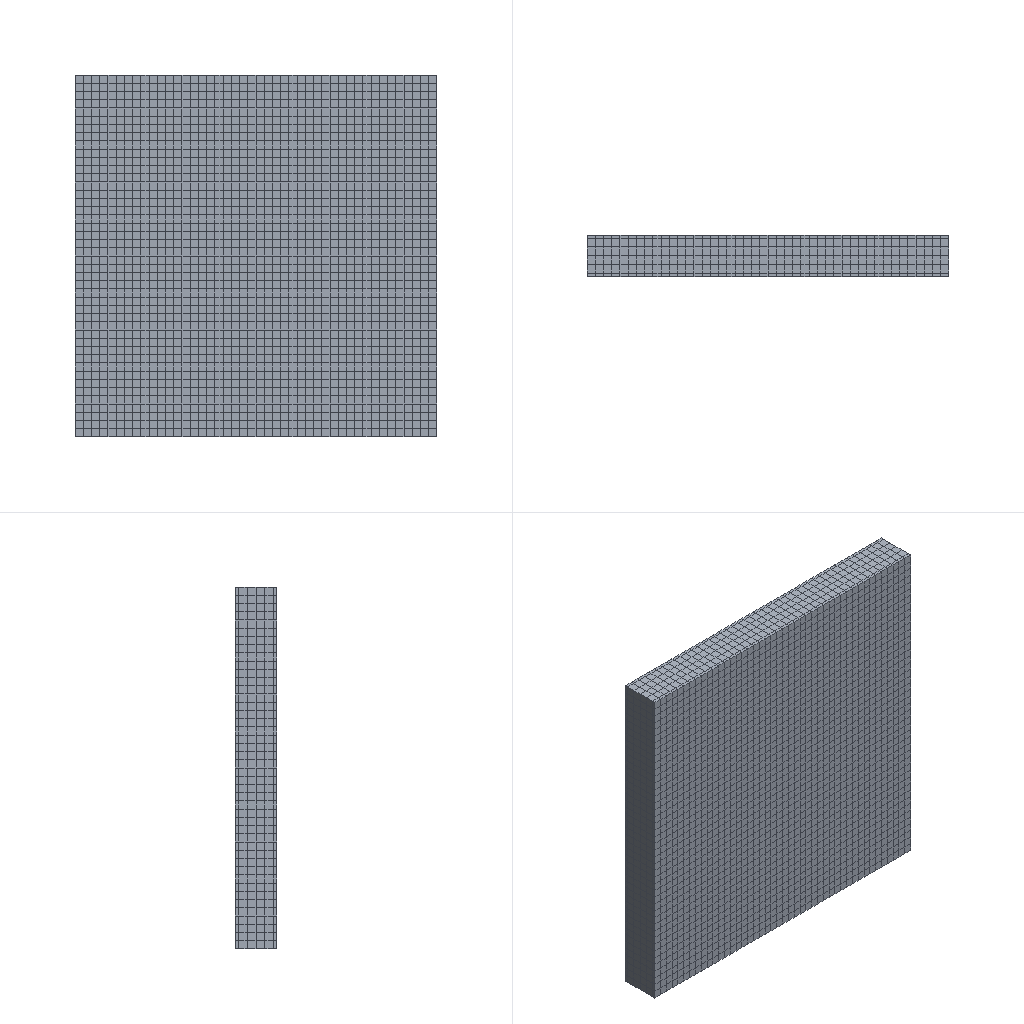Simulation study | abaqus
Set-up summary:
category,name,step,type,value,unit,region
solver,abaqus
solver,version,,,Abaqus/Standard 3DEXPERIENCE R2017x
units,not stated in the deck,,not stated
analysis,deck,,static,static
load_step,Step-all-delete,Step-all-delete,static,nlgeom=True
load_step,Step-insert1,Step-insert1,static,nlgeom=True
load_step,Step-hold1,Step-hold1,static,nlgeom=True
contact,interactions,,,general=0 pairs=0 ties=0
load_step,requested,,,3
mesh,nodes,,,14175
mesh,elements,,,11616
element_type,C3D8R,,solid,11616
load,load commands in deck,,count,4
bc,support commands in deck,,count,1
material,M1,,in results
material,M2,,in results
material,M3,,in results
material,M4,,in results
material,M5,,in results
material,M6,,in results
material,M7,,in results
material,M8,,in results
material,M9,,in results
check,setup vs results,,match,"per instance, exact: element labels, types and connectivity; labels of the nodes the elements use; coordinates of those nodes at SINGLE_PRECISION in 1 of 1 instance(s)"
Abaqus input file, long lists of numbers shortened:
*Heading
** Job name: Job-4 Model name: Model-2-s
** Generated by: Abaqus/CAE 2017
*Preprint, echo=NO, model=NO, history=NO, contact=NO
**
** PARTS
**
*Part, name=Part-1
*Node
      1,           0.,   8.3,          35.
      2,           0.,   8.3,           0.
** (14173 more lines like these left out)
*Element, type=C3D8R
   1,  274,  717, 2566,  189,    1,   17,  102,    4
   2,  717,  718, 2567, 2566,   17,   18,  101,  102
** (11614 more lines like these left out)
*Nset, nset=Set-4
    9,   10,   11,   12,   13,   14,   15,   16,  361,  362,  363,  364,  365,  366,  367,  368
  369,  370,  371,  372,  373,  374,  375,  376,  377,  378,  379,  380,  381,  382,  383,  384
** (252 more lines like these left out)
*Elset, elset=Set-4, generate
 1937,  3872,     1
*Nset, nset=Set-5
     1,     2,     5,     8,     9,    10,    13,    16,    17,    18,    19,    20,    21,    22,    23,    24
    25,    26,    27,    28,    29,    30,    31,    32,    33,    34,    35,    36,    37,    38,    39,    40
** (631 more lines like these left out)
*Elset, elset=Set-5, generate
  3873,  11616,      1
*Nset, nset=Set-3
     1,     2,     5,     8,     9,    10,    11,    12,    13,    14,    15,    16,    17,    18,    19,    20
    21,    22,    23,    24,    25,    26,    27,    28,    29,    30,    31,    32,    33,    34,    35,    36
** (758 more lines like these left out)
*Elset, elset=Set-3, generate
  1937,  11616,      1
*Nset, nset=Set-13
    9,   10,   11,   12,   13,   14,   15,   16,  361,  362,  363,  364,  365,  366,  367,  368
  369,  370,  371,  372,  373,  374,  375,  376,  377,  378,  379,  380,  381,  382,  383,  384
** (252 more lines like these left out)
*Elset, elset=Set-13, generate
 1937,  3872,     1
*Nset, nset=Set-14
     1,     2,     5,     8,     9,    10,    13,    16,    17,    18,    19,    20,    21,    22,    23,    24
    25,    26,    27,    28,    29,    30,    31,    32,    33,    34,    35,    36,    37,    38,    39,    40
** (631 more lines like these left out)
*Elset, elset=Set-14, generate
  3873,  11616,      1
*Nset, nset=Set-15
    1,    2,    3,    4,    5,    6,    7,    8,   17,   18,   19,   20,   21,   22,   23,   24
   25,   26,   27,   28,   29,   30,   31,   32,   33,   34,   35,   36,   37,   38,   39,   40
** (252 more lines like these left out)
*Elset, elset=Set-15, generate
    1,  1936,     1
** Section: M3
*Solid Section, elset=Set-15, material=M3
,
** Section: M1
*Solid Section, elset=Set-13, material=M1
,
** Section: M2
*Solid Section, elset=Set-14, material=M2
,
*End Part
**
**
** ASSEMBLY
**
*Assembly, name=Assembly
**
*Instance, name=Part-1-1, part=Part-1
          0.,          -8.,           0.
*End Instance
**
*Nset, nset=Set-7, instance=Part-1-1, generate
     1,  14175,      1
*Elset, elset=Set-7, instance=Part-1-1, generate
     1,  11616,      1
*Nset, nset=Set-8, instance=Part-1-1, generate
     1,  14175,      1
*Elset, elset=Set-8, instance=Part-1-1, generate
     1,  11616,      1
*Nset, nset=Set-9, instance=Part-1-1, generate
     1,  14175,      1
*Elset, elset=Set-9, instance=Part-1-1, generate
     1,  11616,      1
*Nset, nset=Set-10, instance=Part-1-1
   11,   12,   14,   15,  404,  405,  406,  407,  408,  409,  410,  411,  412,  413,  414,  415
  416,  417,  418,  419,  420,  421,  422,  423,  424,  425,  426,  427,  428,  429,  430,  431
** (125 more lines like these left out)
*Elset, elset=Set-10, instance=Part-1-1, generate
 1937,  3872,     1
*Nset, nset=Set-11, instance=Part-1-1, generate
     1,  14175,      1
*Elset, elset=Set-11, instance=Part-1-1, generate
     1,  11616,      1
*Nset, nset=all, instance=Part-1-1
     1,     2,     5,     8,     9,    10,    11,    12,    13,    14,    15,    16,    17,    18,    19,    20
    21,    22,    23,    24,    25,    26,    27,    28,    29,    30,    31,    32,    33,    34,    35,    36
** (758 more lines like these left out)
*Elset, elset=all, instance=Part-1-1, generate
  1937,  11616,      1
*Nset, nset=bot, instance=Part-1-1
    3,    4,    6,    7,   60,   61,   62,   63,   64,   65,   66,   67,   68,   69,   70,   71
   72,   73,   74,   75,   76,   77,   78,   79,   80,   81,   82,   83,   84,   85,   86,   87
** (125 more lines like these left out)
*Elset, elset=bot, instance=Part-1-1, generate
    1,  1936,     1
*Elset, elset=_Surf-3_S5, internal, instance=Part-1-1, generate
 1937,  3872,     1
*Surface, type=ELEMENT, name=Surf-3
_Surf-3_S5, S5
*Elset, elset=_Surf-6_S2, internal, instance=Part-1-1
    1,    2,    3,    4,    5,    6,    7,    8,    9,   10,   11,   12,   13,   14,   15,   16
   17,   18,   19,   20,   21,   22,   23,   24,   25,   26,   27,   28,   29,   30,   31,   32
** (15 more lines like these left out)
*Elset, elset=_Surf-6_S4, internal, instance=Part-1-1, generate
    44,  11616,     44
*Elset, elset=_Surf-6_S1, internal, instance=Part-1-1
  1893,  1894,  1895,  1896,  1897,  1898,  1899,  1900,  1901,  1902,  1903,  1904,  1905,  1906,  1907,  1908
  1909,  1910,  1911,  1912,  1913,  1914,  1915,  1916,  1917,  1918,  1919,  1920,  1921,  1922,  1923,  1924
** (15 more lines like these left out)
*Elset, elset=_Surf-6_S6, internal, instance=Part-1-1, generate
     1,  11573,     44
*Elset, elset=_Surf-6_S5, internal, instance=Part-1-1, generate
    1,  3872,     1
*Surface, type=ELEMENT, name=Surf-6
_Surf-6_S2, S2
_Surf-6_S4, S4
_Surf-6_S6, S6
_Surf-6_S1, S1
_Surf-6_S5, S5
*Elset, elset=_Surf-7_S5, internal, instance=Part-1-1, generate
 1937,  3872,     1
*Surface, type=ELEMENT, name=Surf-7
_Surf-7_S5, S5
*Elset, elset=_Surf-8_S2, internal, instance=Part-1-1
    1,    2,    3,    4,    5,    6,    7,    8,    9,   10,   11,   12,   13,   14,   15,   16
   17,   18,   19,   20,   21,   22,   23,   24,   25,   26,   27,   28,   29,   30,   31,   32
** (15 more lines like these left out)
*Elset, elset=_Surf-8_S4, internal, instance=Part-1-1, generate
    44,  11616,     44
*Elset, elset=_Surf-8_S1, internal, instance=Part-1-1
  1893,  1894,  1895,  1896,  1897,  1898,  1899,  1900,  1901,  1902,  1903,  1904,  1905,  1906,  1907,  1908
  1909,  1910,  1911,  1912,  1913,  1914,  1915,  1916,  1917,  1918,  1919,  1920,  1921,  1922,  1923,  1924
** (15 more lines like these left out)
*Elset, elset=_Surf-8_S6, internal, instance=Part-1-1, generate
     1,  11573,     44
*Elset, elset=_Surf-8_S5, internal, instance=Part-1-1, generate
    1,  1936,     1
*Surface, type=ELEMENT, name=Surf-8
_Surf-8_S2, S2
_Surf-8_S4, S4
_Surf-8_S6, S6
_Surf-8_S1, S1
_Surf-8_S5, S5
*Elset, elset=_out_surf_S1, internal, instance=Part-1-1
  3829,  3830,  3831,  3832,  3833,  3834,  3835,  3836,  3837,  3838,  3839,  3840,  3841,  3842,  3843,  3844
  3845,  3846,  3847,  3848,  3849,  3850,  3851,  3852,  3853,  3854,  3855,  3856,  3857,  3858,  3859,  3860
** (12 more lines like these left out)
*Elset, elset=_out_surf_S6, internal, instance=Part-1-1, generate
     1,  11573,     44
*Elset, elset=_out_surf_S2, internal, instance=Part-1-1
 1937, 1938, 1939, 1940, 1941, 1942, 1943, 1944, 1945, 1946, 1947, 1948, 1949, 1950, 1951, 1952
 1953, 1954, 1955, 1956, 1957, 1958, 1959, 1960, 1961, 1962, 1963, 1964, 1965, 1966, 1967, 1968
** (12 more lines like these left out)
*Elset, elset=_out_surf_S4, internal, instance=Part-1-1, generate
  1980,  11616,     44
*Elset, elset=_out_surf_S5, internal, instance=Part-1-1, generate
    1,  1936,     1
*Surface, type=ELEMENT, name=out_surf
_out_surf_S1, S1
_out_surf_S6, S6
_out_surf_S2, S2
_out_surf_S4, S4
_out_surf_S5, S5
*End Assembly
**
** MATERIALS
**
*Material, name=M1
*Conductivity
9000.,
*Density
2400.,
*Depvar
      1,
*Elastic
 3.2e+10, 0.23
*Expansion
 1e-05,
*Heat Generation
*Specific Heat
960.,
*User Defined Field
*Material, name=M2
*Conductivity
9000.,
*Density
2400.,
*Depvar
      1,
*Elastic
 3.2e+10, 0.23
*Expansion
 1e-05,
*Heat Generation
*Specific Heat
960.,
*User Defined Field
*Material, name=M3
*Conductivity
9000.,
*Density
2400.,
*Depvar
      1,
*Elastic
 3.2e+10, 0.23
*Expansion
 1e-05,
*Heat Generation
*Specific Heat
960.,
*User Defined Field
*Material, name=M4
*Conductivity
9000.,
*Density
2400.,
*Depvar
      1,
*Heat Generation
*Specific Heat
960.,
*User Defined Field
*Material, name=M5
*Conductivity
9000.,
*Density
2400.,
*Depvar
      1,
*Heat Generation
*Specific Heat
960.,
*User Defined Field
*Material, name=M6
*Conductivity
9000.,
*Density
2400.,
*Depvar
      1,
*Heat Generation
*Specific Heat
960.,
*User Defined Field
*Material, name=M7
*Conductivity
9000.,
*Density
2400.,
*Depvar
      1,
*Heat Generation
*Specific Heat
960.,
*User Defined Field
*Material, name=M8
*Conductivity
9000.,
*Density
2400.,
*Depvar
      1,
*Heat Generation
*Specific Heat
960.,
*User Defined Field
*Material, name=M9
*Conductivity
9000.,
*Density
2400.,
*Depvar
      1,
*Heat Generation
*Specific Heat
960.,
*User Defined Field
**
** PREDEFINED FIELDS
**
** Name: temp   Type: Temperature
*Initial Conditions, type=TEMPERATURE
Set-8, 20.
** ----------------------------------------------------------------
**
** STEP: Step-all-delete
**
*Step, name=Step-all-delete, nlgeom=YES
*Static
1e-08, 1e-08, 1e-13, 1e-08
**
** INTERACTIONS
**
** Interaction: all_delete
*Model Change, remove
Set-7,
**
** OUTPUT REQUESTS
**
*Restart, write, frequency=0
**
** FIELD OUTPUT: F-Output-1
**
*Output, field
*Node Output
CF, NT, RF, RM, RT, U, V
*Element Output, directions=YES
ALPHAN, E, FV, LE, MISES, MISESMAX, MISESONLY, PEEQ, PEEQMAX, PEEQT, PEMAG, PRESSONLY, S, SDV, SF, SSAVG
TEMP, TSHR
*Output, history, frequency=0
*End Step
** ----------------------------------------------------------------
**
** STEP: Step-insert1
**
*Step, name=Step-insert1, nlgeom=YES
*Static
1e-08, 1e-08, 1e-13, 1e-08
**
** INTERACTIONS
**
** Interaction: insert1
*Model Change, add
Set-9,
**
** OUTPUT REQUESTS
**
*Restart, write, frequency=0
**
** FIELD OUTPUT: F-Output-1
**
*Output, field
*Node Output
CF, NT, RF, RM, RT, U, V
*Element Output, directions=YES
ALPHAN, E, FV, LE, MISES, MISESMAX, MISESONLY, PEEQ, PEEQMAX, PEEQT, PEMAG, PRESSONLY, S, SDV, SF, SSAVG
TEMP, TSHR
*Output, history, frequency=0
*End Step
** ----------------------------------------------------------------
**
** STEP: Step-hold1
**
*Step, name=Step-hold1, nlgeom=YES, inc=10000
*Static, stabilize=0.0002, allsdtol=0.05, continue=NO
1., 120., 0.00012, 1.2
**
** BOUNDARY CONDITIONS
**
** Name: BC-2 Type: 位移/转角
*Boundary
Set-10, 2, 2
**
** PREDEFINED FIELDS
**
** Name: Predefined Field-2   Type: Temperature
*Temperature, file=D:\ShuiHuaReYiZhiJi\model\Job-3.odb, bstep=3, binc=1, estep=3, einc=28
**
** OUTPUT REQUESTS
**
*Restart, write, frequency=0
**
** FIELD OUTPUT: F-Output-1
**
*Output, field
*Node Output
CF, NT, RF, RM, RT, U, V
*Element Output, directions=YES
ALPHAN, E, FV, LE, MISES, MISESMAX, MISESONLY, PEEQ, PEEQMAX, PEEQT, PEMAG, PRESSONLY, S, SDV, SF, SSAVG
TEMP, TSHR
*Output, history, frequency=0
*End Step
Results summary:
result,step,,completed,increments=1 time=1e-08/1e-08
result,step,,completed,increments=1 time=1e-08/1e-08
result,step,,completed,increments=101 time=120.0/120.0
result,analysis,,,static
result,last_loadstep,,,3
result,analysis steps,,count,3
result,primary field,,,U
result,reaction total,,FX,0.0,model units
result,reaction total,,FY,-5.537,model units
result,reaction total,,FZ,0.0,model units